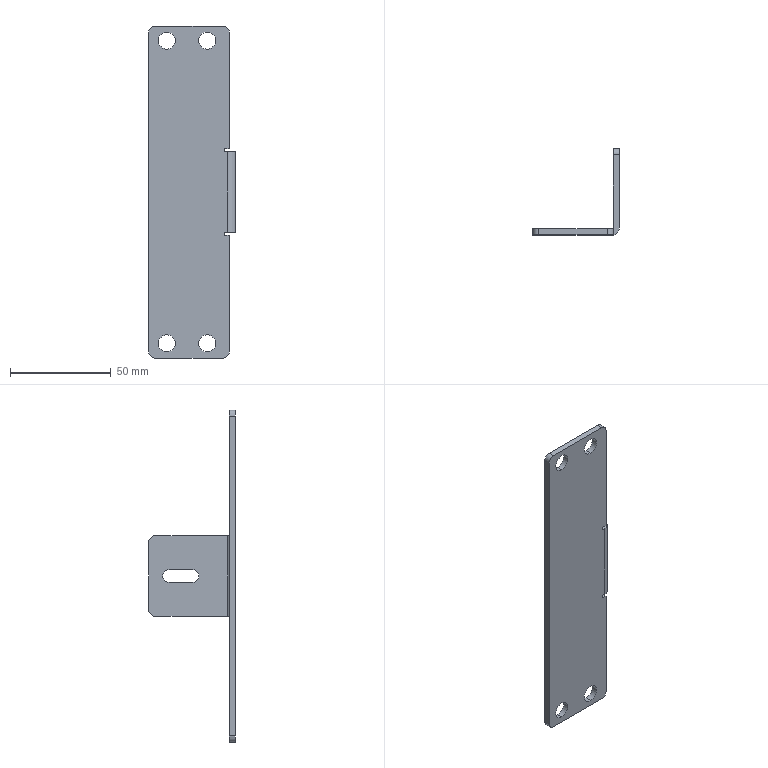Part | SolidWorks | features BaseBody 1 | 1 solid | 37 faces | box 43 x 43 x 165 mm | volume 23785 mm3 | cylinder 19 | plane 18 | commonest cylinder face diameters 8.5 x8 6 x6 6.5 x3 1.473 x1 7.473 x1
STEP:
#1=CARTESIAN_POINT('',(-11.,-3.,71.));
#2=VERTEX_POINT('',#1);
#3=CARTESIAN_POINT('',(-11.,-3.,79.5));
#4=VERTEX_POINT('',#3);
#5=CARTESIAN_POINT('',(-11.,-3.,75.25));
#6=DIRECTION('',(0.,1.,0.));
#7=DIRECTION('',(0.,0.,1.));
#8=AXIS2_PLACEMENT_3D('',#5,#6,#7);
#9=CIRCLE('',#8,4.25);
#10=EDGE_CURVE('',#2,#4,#9,.T.);
#11=ORIENTED_EDGE('',*,*,#10,.F.);
#12=CARTESIAN_POINT('',(-11.,0.,71.));
#13=VERTEX_POINT('',#12);
#14=CARTESIAN_POINT('',(-11.,-10.,71.));
#15=DIRECTION('',(0.,1.,0.));
#16=VECTOR('',#15,1000.);
#17=LINE('',#14,#16);
#18=EDGE_CURVE('',#2,#13,#17,.T.);
#19=ORIENTED_EDGE('',*,*,#18,.T.);
#20=CARTESIAN_POINT('',(-11.,0.,79.5));
#21=VERTEX_POINT('',#20);
#22=CARTESIAN_POINT('',(-11.,0.,75.25));
#23=DIRECTION('',(0.,1.,0.));
#24=DIRECTION('',(0.,0.,1.));
#25=AXIS2_PLACEMENT_3D('',#22,#23,#24);
#26=CIRCLE('',#25,4.25);
#27=EDGE_CURVE('',#13,#21,#26,.T.);
#28=ORIENTED_EDGE('',*,*,#27,.T.);
#29=CARTESIAN_POINT('',(-11.,-10.,79.5));
#30=DIRECTION('',(0.,1.,0.));
#31=VECTOR('',#30,1000.);
#32=LINE('',#29,#31);
#33=EDGE_CURVE('',#4,#21,#32,.T.);
#34=ORIENTED_EDGE('',*,*,#33,.F.);
#35=EDGE_LOOP('',(#11,#19,#28,#34));
#36=FACE_OUTER_BOUND('',#35,.T.);
#37=CARTESIAN_POINT('',(-11.,-10.,75.25));
#38=DIRECTION('',(0.,1.,0.));
#39=DIRECTION('',(0.,0.,1.));
#40=AXIS2_PLACEMENT_3D('',#37,#38,#39);
#41=CYLINDRICAL_SURFACE('',#40,4.25);
#42=ADVANCED_FACE('',(#36),#41,.F.);
#43=CARTESIAN_POINT('',(9.,-3.,71.));
#44=VERTEX_POINT('',#43);
#45=CARTESIAN_POINT('',(9.,-3.,79.5));
#46=VERTEX_POINT('',#45);
#47=CARTESIAN_POINT('',(9.,-3.,75.25));
#48=DIRECTION('',(0.,1.,0.));
#49=DIRECTION('',(0.,0.,1.));
#50=AXIS2_PLACEMENT_3D('',#47,#48,#49);
#51=CIRCLE('',#50,4.25);
#52=EDGE_CURVE('',#44,#46,#51,.T.);
#53=ORIENTED_EDGE('',*,*,#52,.F.);
#54=CARTESIAN_POINT('',(9.,0.,71.));
#55=VERTEX_POINT('',#54);
#56=CARTESIAN_POINT('',(9.,-10.,71.));
#57=DIRECTION('',(0.,1.,0.));
#58=VECTOR('',#57,1000.);
#59=LINE('',#56,#58);
#60=EDGE_CURVE('',#44,#55,#59,.T.);
#61=ORIENTED_EDGE('',*,*,#60,.T.);
#62=CARTESIAN_POINT('',(9.,0.,79.5));
#63=VERTEX_POINT('',#62);
#64=CARTESIAN_POINT('',(9.,0.,75.25));
#65=DIRECTION('',(0.,1.,0.));
#66=DIRECTION('',(0.,0.,1.));
#67=AXIS2_PLACEMENT_3D('',#64,#65,#66);
#68=CIRCLE('',#67,4.25);
#69=EDGE_CURVE('',#55,#63,#68,.T.);
#70=ORIENTED_EDGE('',*,*,#69,.T.);
#71=CARTESIAN_POINT('',(9.,-10.,79.5));
#72=DIRECTION('',(0.,1.,0.));
#73=VECTOR('',#72,1000.);
#74=LINE('',#71,#73);
#75=EDGE_CURVE('',#46,#63,#74,.T.);
#76=ORIENTED_EDGE('',*,*,#75,.F.);
#77=EDGE_LOOP('',(#53,#61,#70,#76));
#78=FACE_OUTER_BOUND('',#77,.T.);
#79=CARTESIAN_POINT('',(9.,-10.,75.25));
#80=DIRECTION('',(0.,1.,0.));
#81=DIRECTION('',(0.,0.,1.));
#82=AXIS2_PLACEMENT_3D('',#79,#80,#81);
#83=CYLINDRICAL_SURFACE('',#82,4.25);
#84=ADVANCED_FACE('',(#78),#83,.F.);
#85=CARTESIAN_POINT('',(9.,-3.,-79.5));
#86=VERTEX_POINT('',#85);
#87=CARTESIAN_POINT('',(9.,-3.,-71.));
#88=VERTEX_POINT('',#87);
#89=CARTESIAN_POINT('',(9.,-3.,-75.25));
#90=DIRECTION('',(0.,1.,0.));
#91=DIRECTION('',(0.,0.,1.));
#92=AXIS2_PLACEMENT_3D('',#89,#90,#91);
#93=CIRCLE('',#92,4.25);
#94=EDGE_CURVE('',#86,#88,#93,.T.);
#95=ORIENTED_EDGE('',*,*,#94,.F.);
#96=CARTESIAN_POINT('',(9.,0.,-79.5));
#97=VERTEX_POINT('',#96);
#98=CARTESIAN_POINT('',(9.,-10.,-79.5));
#99=DIRECTION('',(0.,1.,0.));
#100=VECTOR('',#99,1000.);
#101=LINE('',#98,#100);
#102=EDGE_CURVE('',#86,#97,#101,.T.);
#103=ORIENTED_EDGE('',*,*,#102,.T.);
#104=CARTESIAN_POINT('',(9.,0.,-71.));
#105=VERTEX_POINT('',#104);
#106=CARTESIAN_POINT('',(9.,0.,-75.25));
#107=DIRECTION('',(0.,1.,0.));
#108=DIRECTION('',(0.,0.,1.));
#109=AXIS2_PLACEMENT_3D('',#106,#107,#108);
#110=CIRCLE('',#109,4.25);
#111=EDGE_CURVE('',#97,#105,#110,.T.);
#112=ORIENTED_EDGE('',*,*,#111,.T.);
#113=CARTESIAN_POINT('',(9.,-10.,-71.));
#114=DIRECTION('',(0.,1.,0.));
#115=VECTOR('',#114,1000.);
#116=LINE('',#113,#115);
#117=EDGE_CURVE('',#88,#105,#116,.T.);
#118=ORIENTED_EDGE('',*,*,#117,.F.);
#119=EDGE_LOOP('',(#95,#103,#112,#118));
#120=FACE_OUTER_BOUND('',#119,.T.);
#121=CARTESIAN_POINT('',(9.,-10.,-75.25));
#122=DIRECTION('',(0.,1.,0.));
#123=DIRECTION('',(0.,0.,1.));
#124=AXIS2_PLACEMENT_3D('',#121,#122,#123);
#125=CYLINDRICAL_SURFACE('',#124,4.25);
#126=ADVANCED_FACE('',(#120),#125,.F.);
#127=CARTESIAN_POINT('',(-11.,-3.,-79.5));
#128=VERTEX_POINT('',#127);
#129=CARTESIAN_POINT('',(-11.,-3.,-71.));
#130=VERTEX_POINT('',#129);
#131=CARTESIAN_POINT('',(-11.,-3.,-75.25));
#132=DIRECTION('',(0.,1.,0.));
#133=DIRECTION('',(0.,0.,1.));
#134=AXIS2_PLACEMENT_3D('',#131,#132,#133);
#135=CIRCLE('',#134,4.25);
#136=EDGE_CURVE('',#128,#130,#135,.T.);
#137=ORIENTED_EDGE('',*,*,#136,.F.);
#138=CARTESIAN_POINT('',(-11.,0.,-79.5));
#139=VERTEX_POINT('',#138);
#140=CARTESIAN_POINT('',(-11.,-10.,-79.5));
#141=DIRECTION('',(0.,1.,0.));
#142=VECTOR('',#141,1000.);
#143=LINE('',#140,#142);
#144=EDGE_CURVE('',#128,#139,#143,.T.);
#145=ORIENTED_EDGE('',*,*,#144,.T.);
#146=CARTESIAN_POINT('',(-11.,0.,-71.));
#147=VERTEX_POINT('',#146);
#148=CARTESIAN_POINT('',(-11.,0.,-75.25));
#149=DIRECTION('',(0.,1.,0.));
#150=DIRECTION('',(0.,0.,1.));
#151=AXIS2_PLACEMENT_3D('',#148,#149,#150);
#152=CIRCLE('',#151,4.25);
#153=EDGE_CURVE('',#139,#147,#152,.T.);
#154=ORIENTED_EDGE('',*,*,#153,.T.);
#155=CARTESIAN_POINT('',(-11.,-10.,-71.));
#156=DIRECTION('',(0.,1.,0.));
#157=VECTOR('',#156,1000.);
#158=LINE('',#155,#157);
#159=EDGE_CURVE('',#130,#147,#158,.T.);
#160=ORIENTED_EDGE('',*,*,#159,.F.);
#161=EDGE_LOOP('',(#137,#145,#154,#160));
#162=FACE_OUTER_BOUND('',#161,.T.);
#163=CARTESIAN_POINT('',(-11.,-10.,-75.25));
#164=DIRECTION('',(0.,1.,0.));
#165=DIRECTION('',(0.,0.,1.));
#166=AXIS2_PLACEMENT_3D('',#163,#164,#165);
#167=CYLINDRICAL_SURFACE('',#166,4.25);
#168=ADVANCED_FACE('',(#162),#167,.F.);
#169=CARTESIAN_POINT('',(20.,33.,0.));
#170=VERTEX_POINT('',#169);
#171=CARTESIAN_POINT('',(20.,29.75,3.25));
#172=VERTEX_POINT('',#171);
#173=CARTESIAN_POINT('',(20.,29.75,0.));
#174=DIRECTION('',(1.,0.,0.));
#175=DIRECTION('',(0.,1.,0.));
#176=AXIS2_PLACEMENT_3D('',#173,#174,#175);
#177=CIRCLE('',#176,3.25);
#178=EDGE_CURVE('',#170,#172,#177,.T.);
#179=ORIENTED_EDGE('',*,*,#178,.F.);
#180=CARTESIAN_POINT('',(23.,33.,0.));
#181=VERTEX_POINT('',#180);
#182=CARTESIAN_POINT('',(13.,33.,0.));
#183=DIRECTION('',(1.,0.,0.));
#184=VECTOR('',#183,1000.);
#185=LINE('',#182,#184);
#186=EDGE_CURVE('',#170,#181,#185,.T.);
#187=ORIENTED_EDGE('',*,*,#186,.T.);
#188=CARTESIAN_POINT('',(23.,29.75,3.25));
#189=VERTEX_POINT('',#188);
#190=CARTESIAN_POINT('',(23.,29.75,0.));
#191=DIRECTION('',(-1.,0.,0.));
#192=DIRECTION('',(0.,1.,0.));
#193=AXIS2_PLACEMENT_3D('',#190,#191,#192);
#194=CIRCLE('',#193,3.25);
#195=EDGE_CURVE('',#189,#181,#194,.T.);
#196=ORIENTED_EDGE('',*,*,#195,.F.);
#197=CARTESIAN_POINT('',(13.,29.75,3.25));
#198=DIRECTION('',(-1.,0.,0.));
#199=VECTOR('',#198,1000.);
#200=LINE('',#197,#199);
#201=EDGE_CURVE('',#189,#172,#200,.T.);
#202=ORIENTED_EDGE('',*,*,#201,.T.);
#203=EDGE_LOOP('',(#179,#187,#196,#202));
#204=FACE_OUTER_BOUND('',#203,.T.);
#205=CARTESIAN_POINT('',(13.,29.75,0.));
#206=DIRECTION('',(1.,0.,0.));
#207=DIRECTION('',(0.,1.,0.));
#208=AXIS2_PLACEMENT_3D('',#205,#206,#207);
#209=CYLINDRICAL_SURFACE('',#208,3.25);
#210=ADVANCED_FACE('',(#204),#209,.F.);
#211=CARTESIAN_POINT('',(17.,0.,-82.5));
#212=VERTEX_POINT('',#211);
#213=CARTESIAN_POINT('',(20.,0.,-79.5));
#214=VERTEX_POINT('',#213);
#215=CARTESIAN_POINT('',(17.,0.,-79.5));
#216=DIRECTION('',(0.,-1.,0.));
#217=DIRECTION('',(0.,0.,1.));
#218=AXIS2_PLACEMENT_3D('',#215,#216,#217);
#219=CIRCLE('',#218,3.);
#220=EDGE_CURVE('',#212,#214,#219,.T.);
#221=ORIENTED_EDGE('',*,*,#220,.F.);
#222=CARTESIAN_POINT('',(-17.,0.,-82.5));
#223=VERTEX_POINT('',#222);
#224=CARTESIAN_POINT('',(0.,0.,-82.5));
#225=DIRECTION('',(1.,0.,0.));
#226=VECTOR('',#225,1000.);
#227=LINE('',#224,#226);
#228=EDGE_CURVE('',#223,#212,#227,.T.);
#229=ORIENTED_EDGE('',*,*,#228,.F.);
#230=CARTESIAN_POINT('',(-20.,0.,-79.5));
#231=VERTEX_POINT('',#230);
#232=CARTESIAN_POINT('',(-17.,0.,-79.5));
#233=DIRECTION('',(0.,-1.,0.));
#234=DIRECTION('',(0.,0.,1.));
#235=AXIS2_PLACEMENT_3D('',#232,#233,#234);
#236=CIRCLE('',#235,3.);
#237=EDGE_CURVE('',#231,#223,#236,.T.);
#238=ORIENTED_EDGE('',*,*,#237,.F.);
#239=CARTESIAN_POINT('',(-20.,0.,79.5));
#240=VERTEX_POINT('',#239);
#241=CARTESIAN_POINT('',(-20.,0.,0.));
#242=DIRECTION('',(0.,0.,-1.));
#243=VECTOR('',#242,1000.);
#244=LINE('',#241,#243);
#245=EDGE_CURVE('',#240,#231,#244,.T.);
#246=ORIENTED_EDGE('',*,*,#245,.F.);
#247=CARTESIAN_POINT('',(-17.,0.,82.5));
#248=VERTEX_POINT('',#247);
#249=CARTESIAN_POINT('',(-17.,0.,79.5));
#250=DIRECTION('',(0.,-1.,0.));
#251=DIRECTION('',(0.,0.,1.));
#252=AXIS2_PLACEMENT_3D('',#249,#250,#251);
#253=CIRCLE('',#252,3.);
#254=EDGE_CURVE('',#248,#240,#253,.T.);
#255=ORIENTED_EDGE('',*,*,#254,.F.);
#256=CARTESIAN_POINT('',(17.,0.,82.5));
#257=VERTEX_POINT('',#256);
#258=CARTESIAN_POINT('',(0.,0.,82.5));
#259=DIRECTION('',(-1.,0.,0.));
#260=VECTOR('',#259,1000.);
#261=LINE('',#258,#260);
#262=EDGE_CURVE('',#257,#248,#261,.T.);
#263=ORIENTED_EDGE('',*,*,#262,.F.);
#264=CARTESIAN_POINT('',(20.,0.,79.5));
#265=VERTEX_POINT('',#264);
#266=CARTESIAN_POINT('',(17.,0.,79.5));
#267=DIRECTION('',(0.,-1.,0.));
#268=DIRECTION('',(0.,0.,1.));
#269=AXIS2_PLACEMENT_3D('',#266,#267,#268);
#270=CIRCLE('',#269,3.);
#271=EDGE_CURVE('',#265,#257,#270,.T.);
#272=ORIENTED_EDGE('',*,*,#271,.F.);
#273=CARTESIAN_POINT('',(20.,0.,21.5));
#274=VERTEX_POINT('',#273);
#275=CARTESIAN_POINT('',(20.,0.,0.));
#276=DIRECTION('',(0.,0.,1.));
#277=VECTOR('',#276,1000.);
#278=LINE('',#275,#277);
#279=EDGE_CURVE('',#274,#265,#278,.T.);
#280=ORIENTED_EDGE('',*,*,#279,.F.);
#281=CARTESIAN_POINT('',(17.763,0.,21.5));
#282=VERTEX_POINT('',#281);
#283=CARTESIAN_POINT('',(0.,0.,21.5));
#284=DIRECTION('',(1.,0.,0.));
#285=VECTOR('',#284,1000.);
#286=LINE('',#283,#285);
#287=EDGE_CURVE('',#282,#274,#286,.T.);
#288=ORIENTED_EDGE('',*,*,#287,.F.);
#289=CARTESIAN_POINT('',(17.763,0.,20.));
#290=VERTEX_POINT('',#289);
#291=CARTESIAN_POINT('',(17.763,0.,20.));
#292=DIRECTION('',(0.,0.,1.));
#293=VECTOR('',#292,1000.);
#294=LINE('',#291,#293);
#295=EDGE_CURVE('',#290,#282,#294,.T.);
#296=ORIENTED_EDGE('',*,*,#295,.F.);
#297=CARTESIAN_POINT('',(19.263,0.,20.));
#298=VERTEX_POINT('',#297);
#299=CARTESIAN_POINT('',(19.263,0.,20.));
#300=DIRECTION('',(-1.,0.,0.));
#301=VECTOR('',#300,1000.);
#302=LINE('',#299,#301);
#303=EDGE_CURVE('',#298,#290,#302,.T.);
#304=ORIENTED_EDGE('',*,*,#303,.F.);
#305=CARTESIAN_POINT('',(19.263,0.,-20.));
#306=VERTEX_POINT('',#305);
#307=CARTESIAN_POINT('',(19.263,0.,0.));
#308=DIRECTION('',(0.,0.,1.));
#309=VECTOR('',#308,1000.);
#310=LINE('',#307,#309);
#311=EDGE_CURVE('',#306,#298,#310,.T.);
#312=ORIENTED_EDGE('',*,*,#311,.F.);
#313=CARTESIAN_POINT('',(17.763,0.,-20.));
#314=VERTEX_POINT('',#313);
#315=CARTESIAN_POINT('',(17.763,0.,-20.));
#316=DIRECTION('',(1.,0.,0.));
#317=VECTOR('',#316,1000.);
#318=LINE('',#315,#317);
#319=EDGE_CURVE('',#314,#306,#318,.T.);
#320=ORIENTED_EDGE('',*,*,#319,.F.);
#321=CARTESIAN_POINT('',(17.763,0.,-21.5));
#322=VERTEX_POINT('',#321);
#323=CARTESIAN_POINT('',(17.763,0.,-21.5));
#324=DIRECTION('',(0.,0.,1.));
#325=VECTOR('',#324,1000.);
#326=LINE('',#323,#325);
#327=EDGE_CURVE('',#322,#314,#326,.T.);
#328=ORIENTED_EDGE('',*,*,#327,.F.);
#329=CARTESIAN_POINT('',(20.,0.,-21.5));
#330=VERTEX_POINT('',#329);
#331=CARTESIAN_POINT('',(0.,0.,-21.5));
#332=DIRECTION('',(-1.,0.,0.));
#333=VECTOR('',#332,1000.);
#334=LINE('',#331,#333);
#335=EDGE_CURVE('',#330,#322,#334,.T.);
#336=ORIENTED_EDGE('',*,*,#335,.F.);
#337=CARTESIAN_POINT('',(20.,0.,0.));
#338=DIRECTION('',(0.,0.,1.));
#339=VECTOR('',#338,1000.);
#340=LINE('',#337,#339);
#341=EDGE_CURVE('',#214,#330,#340,.T.);
#342=ORIENTED_EDGE('',*,*,#341,.F.);
#343=EDGE_LOOP('',(#221,#229,#238,#246,#255,#263,#272,#280,#288,#296,#304,#312,#320,#328,#336,#342));
#344=FACE_OUTER_BOUND('',#343,.T.);
#345=CARTESIAN_POINT('',(-11.,0.,75.25));
#346=DIRECTION('',(0.,1.,0.));
#347=DIRECTION('',(0.,0.,1.));
#348=AXIS2_PLACEMENT_3D('',#345,#346,#347);
#349=CIRCLE('',#348,4.25);
#350=EDGE_CURVE('',#21,#13,#349,.T.);
#351=ORIENTED_EDGE('',*,*,#350,.F.);
#352=ORIENTED_EDGE('',*,*,#27,.F.);
#353=EDGE_LOOP('',(#351,#352));
#354=FACE_BOUND('',#353,.T.);
#355=CARTESIAN_POINT('',(9.,0.,75.25));
#356=DIRECTION('',(0.,1.,0.));
#357=DIRECTION('',(0.,0.,1.));
#358=AXIS2_PLACEMENT_3D('',#355,#356,#357);
#359=CIRCLE('',#358,4.25);
#360=EDGE_CURVE('',#63,#55,#359,.T.);
#361=ORIENTED_EDGE('',*,*,#360,.F.);
#362=ORIENTED_EDGE('',*,*,#69,.F.);
#363=EDGE_LOOP('',(#361,#362));
#364=FACE_BOUND('',#363,.T.);
#365=CARTESIAN_POINT('',(9.,0.,-75.25));
#366=DIRECTION('',(0.,1.,0.));
#367=DIRECTION('',(0.,0.,1.));
#368=AXIS2_PLACEMENT_3D('',#365,#366,#367);
#369=CIRCLE('',#368,4.25);
#370=EDGE_CURVE('',#105,#97,#369,.T.);
#371=ORIENTED_EDGE('',*,*,#370,.F.);
#372=ORIENTED_EDGE('',*,*,#111,.F.);
#373=EDGE_LOOP('',(#371,#372));
#374=FACE_BOUND('',#373,.T.);
#375=CARTESIAN_POINT('',(-11.,0.,-75.25));
#376=DIRECTION('',(0.,1.,0.));
#377=DIRECTION('',(0.,0.,1.));
#378=AXIS2_PLACEMENT_3D('',#375,#376,#377);
#379=CIRCLE('',#378,4.25);
#380=EDGE_CURVE('',#147,#139,#379,.T.);
#381=ORIENTED_EDGE('',*,*,#380,.F.);
#382=ORIENTED_EDGE('',*,*,#153,.F.);
#383=EDGE_LOOP('',(#381,#382));
#384=FACE_BOUND('',#383,.T.);
#385=CARTESIAN_POINT('',(0.,0.,0.));
#386=DIRECTION('',(0.,-1.,0.));
#387=DIRECTION('',(0.,0.,-1.));
#388=AXIS2_PLACEMENT_3D('',#385,#386,#387);
#389=PLANE('',#388);
#390=ADVANCED_FACE('',(#344,#354,#364,#374,#384),#389,.F.);
#391=ORIENTED_EDGE('',*,*,#341,.T.);
#392=CARTESIAN_POINT('',(20.,-3.,-21.5));
#393=VERTEX_POINT('',#392);
#394=CARTESIAN_POINT('',(20.,-3.,-21.5));
#395=DIRECTION('',(0.,-1.,0.));
#396=VECTOR('',#395,1000.);
#397=LINE('',#394,#396);
#398=EDGE_CURVE('',#330,#393,#397,.T.);
#399=ORIENTED_EDGE('',*,*,#398,.T.);
#400=CARTESIAN_POINT('',(20.,-3.,-79.5));
#401=VERTEX_POINT('',#400);
#402=CARTESIAN_POINT('',(20.,-3.,82.5));
#403=DIRECTION('',(0.,0.,-1.));
#404=VECTOR('',#403,1000.);
#405=LINE('',#402,#404);
#406=EDGE_CURVE('',#393,#401,#405,.T.);
#407=ORIENTED_EDGE('',*,*,#406,.T.);
#408=CARTESIAN_POINT('',(20.,-3.,-79.5));
#409=DIRECTION('',(0.,1.,0.));
#410=VECTOR('',#409,1000.);
#411=LINE('',#408,#410);
#412=EDGE_CURVE('',#401,#214,#411,.T.);
#413=ORIENTED_EDGE('',*,*,#412,.T.);
#414=EDGE_LOOP('',(#391,#399,#407,#413));
#415=FACE_OUTER_BOUND('',#414,.T.);
#416=CARTESIAN_POINT('',(20.,-3.,82.5));
#417=DIRECTION('',(1.,0.,0.));
#418=DIRECTION('',(0.,0.,-1.));
#419=AXIS2_PLACEMENT_3D('',#416,#417,#418);
#420=PLANE('',#419);
#421=ADVANCED_FACE('',(#415),#420,.T.);
#422=ORIENTED_EDGE('',*,*,#220,.T.);
#423=ORIENTED_EDGE('',*,*,#412,.F.);
#424=CARTESIAN_POINT('',(17.,-3.,-82.5));
#425=VERTEX_POINT('',#424);
#426=CARTESIAN_POINT('',(17.,-3.,-79.5));
#427=DIRECTION('',(0.,1.,0.));
#428=DIRECTION('',(0.,0.,1.));
#429=AXIS2_PLACEMENT_3D('',#426,#427,#428);
#430=CIRCLE('',#429,3.);
#431=EDGE_CURVE('',#401,#425,#430,.T.);
#432=ORIENTED_EDGE('',*,*,#431,.T.);
#433=CARTESIAN_POINT('',(17.,-3.,-82.5));
#434=DIRECTION('',(0.,1.,0.));
#435=VECTOR('',#434,1000.);
#436=LINE('',#433,#435);
#437=EDGE_CURVE('',#425,#212,#436,.T.);
#438=ORIENTED_EDGE('',*,*,#437,.T.);
#439=EDGE_LOOP('',(#422,#423,#432,#438));
#440=FACE_OUTER_BOUND('',#439,.T.);
#441=CARTESIAN_POINT('',(17.,-3.,-79.5));
#442=DIRECTION('',(0.,1.,0.));
#443=DIRECTION('',(0.,0.,1.));
#444=AXIS2_PLACEMENT_3D('',#441,#442,#443);
#445=CYLINDRICAL_SURFACE('',#444,3.);
#446=ADVANCED_FACE('',(#440),#445,.T.);
#447=CARTESIAN_POINT('',(-17.,-3.,-82.5));
#448=VERTEX_POINT('',#447);
#449=CARTESIAN_POINT('',(-20.,-3.,-82.5));
#450=DIRECTION('',(-1.,0.,0.));
#451=VECTOR('',#450,1000.);
#452=LINE('',#449,#451);
#453=EDGE_CURVE('',#425,#448,#452,.T.);
#454=ORIENTED_EDGE('',*,*,#453,.T.);
#455=CARTESIAN_POINT('',(-17.,-3.,-82.5));
#456=DIRECTION('',(0.,1.,0.));
#457=VECTOR('',#456,1000.);
#458=LINE('',#455,#457);
#459=EDGE_CURVE('',#448,#223,#458,.T.);
#460=ORIENTED_EDGE('',*,*,#459,.T.);
#461=ORIENTED_EDGE('',*,*,#228,.T.);
#462=ORIENTED_EDGE('',*,*,#437,.F.);
#463=EDGE_LOOP('',(#454,#460,#461,#462));
#464=FACE_OUTER_BOUND('',#463,.T.);
#465=CARTESIAN_POINT('',(-20.,-3.,-82.5));
#466=DIRECTION('',(0.,0.,-1.));
#467=DIRECTION('',(-1.,0.,0.));
#468=AXIS2_PLACEMENT_3D('',#465,#466,#467);
#469=PLANE('',#468);
#470=ADVANCED_FACE('',(#464),#469,.T.);
#471=ORIENTED_EDGE('',*,*,#237,.T.);
#472=ORIENTED_EDGE('',*,*,#459,.F.);
#473=CARTESIAN_POINT('',(-20.,-3.,-79.5));
#474=VERTEX_POINT('',#473);
#475=CARTESIAN_POINT('',(-17.,-3.,-79.5));
#476=DIRECTION('',(0.,1.,0.));
#477=DIRECTION('',(0.,0.,1.));
#478=AXIS2_PLACEMENT_3D('',#475,#476,#477);
#479=CIRCLE('',#478,3.);
#480=EDGE_CURVE('',#448,#474,#479,.T.);
#481=ORIENTED_EDGE('',*,*,#480,.T.);
#482=CARTESIAN_POINT('',(-20.,-3.,-79.5));
#483=DIRECTION('',(0.,1.,0.));
#484=VECTOR('',#483,1000.);
#485=LINE('',#482,#484);
#486=EDGE_CURVE('',#474,#231,#485,.T.);
#487=ORIENTED_EDGE('',*,*,#486,.T.);
#488=EDGE_LOOP('',(#471,#472,#481,#487));
#489=FACE_OUTER_BOUND('',#488,.T.);
#490=CARTESIAN_POINT('',(-17.,-3.,-79.5));
#491=DIRECTION('',(0.,1.,0.));
#492=DIRECTION('',(0.,0.,1.));
#493=AXIS2_PLACEMENT_3D('',#490,#491,#492);
#494=CYLINDRICAL_SURFACE('',#493,3.);
#495=ADVANCED_FACE('',(#489),#494,.T.);
#496=CARTESIAN_POINT('',(-20.,-3.,79.5));
#497=VERTEX_POINT('',#496);
#498=CARTESIAN_POINT('',(-20.,-3.,82.5));
#499=DIRECTION('',(0.,0.,1.));
#500=VECTOR('',#499,1000.);
#501=LINE('',#498,#500);
#502=EDGE_CURVE('',#474,#497,#501,.T.);
#503=ORIENTED_EDGE('',*,*,#502,.T.);
#504=CARTESIAN_POINT('',(-20.,-3.,79.5));
#505=DIRECTION('',(0.,1.,0.));
#506=VECTOR('',#505,1000.);
#507=LINE('',#504,#506);
#508=EDGE_CURVE('',#497,#240,#507,.T.);
#509=ORIENTED_EDGE('',*,*,#508,.T.);
#510=ORIENTED_EDGE('',*,*,#245,.T.);
#511=ORIENTED_EDGE('',*,*,#486,.F.);
#512=EDGE_LOOP('',(#503,#509,#510,#511));
#513=FACE_OUTER_BOUND('',#512,.T.);
#514=CARTESIAN_POINT('',(-20.,-3.,82.5));
#515=DIRECTION('',(-1.,0.,0.));
#516=DIRECTION('',(0.,0.,1.));
#517=AXIS2_PLACEMENT_3D('',#514,#515,#516);
#518=PLANE('',#517);
#519=ADVANCED_FACE('',(#513),#518,.T.);
#520=ORIENTED_EDGE('',*,*,#254,.T.);
#521=ORIENTED_EDGE('',*,*,#508,.F.);
#522=CARTESIAN_POINT('',(-17.,-3.,82.5));
#523=VERTEX_POINT('',#522);
#524=CARTESIAN_POINT('',(-17.,-3.,79.5));
#525=DIRECTION('',(0.,1.,0.));
#526=DIRECTION('',(0.,0.,1.));
#527=AXIS2_PLACEMENT_3D('',#524,#525,#526);
#528=CIRCLE('',#527,3.);
#529=EDGE_CURVE('',#497,#523,#528,.T.);
#530=ORIENTED_EDGE('',*,*,#529,.T.);
#531=CARTESIAN_POINT('',(-17.,-3.,82.5));
#532=DIRECTION('',(0.,1.,0.));
#533=VECTOR('',#532,1000.);
#534=LINE('',#531,#533);
#535=EDGE_CURVE('',#523,#248,#534,.T.);
#536=ORIENTED_EDGE('',*,*,#535,.T.);
#537=EDGE_LOOP('',(#520,#521,#530,#536));
#538=FACE_OUTER_BOUND('',#537,.T.);
#539=CARTESIAN_POINT('',(-17.,-3.,79.5));
#540=DIRECTION('',(0.,1.,0.));
#541=DIRECTION('',(0.,0.,1.));
#542=AXIS2_PLACEMENT_3D('',#539,#540,#541);
#543=CYLINDRICAL_SURFACE('',#542,3.);
#544=ADVANCED_FACE('',(#538),#543,.T.);
#545=CARTESIAN_POINT('',(17.,-3.,82.5));
#546=VERTEX_POINT('',#545);
#547=CARTESIAN_POINT('',(-20.,-3.,82.5));
#548=DIRECTION('',(1.,0.,0.));
#549=VECTOR('',#548,1000.);
#550=LINE('',#547,#549);
#551=EDGE_CURVE('',#523,#546,#550,.T.);
#552=ORIENTED_EDGE('',*,*,#551,.T.);
#553=CARTESIAN_POINT('',(17.,-3.,82.5));
#554=DIRECTION('',(0.,1.,0.));
#555=VECTOR('',#554,1000.);
#556=LINE('',#553,#555);
#557=EDGE_CURVE('',#546,#257,#556,.T.);
#558=ORIENTED_EDGE('',*,*,#557,.T.);
#559=ORIENTED_EDGE('',*,*,#262,.T.);
#560=ORIENTED_EDGE('',*,*,#535,.F.);
#561=EDGE_LOOP('',(#552,#558,#559,#560));
#562=FACE_OUTER_BOUND('',#561,.T.);
#563=CARTESIAN_POINT('',(-20.,-3.,82.5));
#564=DIRECTION('',(0.,0.,1.));
#565=DIRECTION('',(1.,0.,0.));
#566=AXIS2_PLACEMENT_3D('',#563,#564,#565);
#567=PLANE('',#566);
#568=ADVANCED_FACE('',(#562),#567,.T.);
#569=ORIENTED_EDGE('',*,*,#271,.T.);
#570=ORIENTED_EDGE('',*,*,#557,.F.);
#571=CARTESIAN_POINT('',(20.,-3.,79.5));
#572=VERTEX_POINT('',#571);
#573=CARTESIAN_POINT('',(17.,-3.,79.5));
#574=DIRECTION('',(0.,1.,0.));
#575=DIRECTION('',(0.,0.,1.));
#576=AXIS2_PLACEMENT_3D('',#573,#574,#575);
#577=CIRCLE('',#576,3.);
#578=EDGE_CURVE('',#546,#572,#577,.T.);
#579=ORIENTED_EDGE('',*,*,#578,.T.);
#580=CARTESIAN_POINT('',(20.,-3.,79.5));
#581=DIRECTION('',(0.,1.,0.));
#582=VECTOR('',#581,1000.);
#583=LINE('',#580,#582);
#584=EDGE_CURVE('',#572,#265,#583,.T.);
#585=ORIENTED_EDGE('',*,*,#584,.T.);
#586=EDGE_LOOP('',(#569,#570,#579,#585));
#587=FACE_OUTER_BOUND('',#586,.T.);
#588=CARTESIAN_POINT('',(17.,-3.,79.5));
#589=DIRECTION('',(0.,1.,0.));
#590=DIRECTION('',(0.,0.,1.));
#591=AXIS2_PLACEMENT_3D('',#588,#589,#590);
#592=CYLINDRICAL_SURFACE('',#591,3.);
#593=ADVANCED_FACE('',(#587),#592,.T.);
#594=CARTESIAN_POINT('',(20.,-3.,21.5));
#595=VERTEX_POINT('',#594);
#596=CARTESIAN_POINT('',(20.,-3.,82.5));
#597=DIRECTION('',(0.,0.,-1.));
#598=VECTOR('',#597,1000.);
#599=LINE('',#596,#598);
#600=EDGE_CURVE('',#572,#595,#599,.T.);
#601=ORIENTED_EDGE('',*,*,#600,.T.);
#602=CARTESIAN_POINT('',(20.,-3.,21.5));
#603=DIRECTION('',(0.,1.,0.));
#604=VECTOR('',#603,1000.);
#605=LINE('',#602,#604);
#606=EDGE_CURVE('',#595,#274,#605,.T.);
#607=ORIENTED_EDGE('',*,*,#606,.T.);
#608=ORIENTED_EDGE('',*,*,#279,.T.);
#609=ORIENTED_EDGE('',*,*,#584,.F.);
#610=EDGE_LOOP('',(#601,#607,#608,#609));
#611=FACE_OUTER_BOUND('',#610,.T.);
#612=CARTESIAN_POINT('',(20.,-3.,82.5));
#613=DIRECTION('',(1.,0.,0.));
#614=DIRECTION('',(0.,0.,-1.));
#615=AXIS2_PLACEMENT_3D('',#612,#613,#614);
#616=PLANE('',#615);
#617=ADVANCED_FACE('',(#611),#616,.T.);
#618=ORIENTED_EDGE('',*,*,#287,.T.);
#619=ORIENTED_EDGE('',*,*,#606,.F.);
#620=CARTESIAN_POINT('',(17.763,-3.,21.5));
#621=VERTEX_POINT('',#620);
#622=CARTESIAN_POINT('',(17.763,-3.,21.5));
#623=DIRECTION('',(-1.,0.,0.));
#624=VECTOR('',#623,1000.);
#625=LINE('',#622,#624);
#626=EDGE_CURVE('',#595,#621,#625,.T.);
#627=ORIENTED_EDGE('',*,*,#626,.T.);
#628=CARTESIAN_POINT('',(17.763,0.,21.5));
#629=DIRECTION('',(0.,1.,0.));
#630=VECTOR('',#629,1000.);
#631=LINE('',#628,#630);
#632=EDGE_CURVE('',#621,#282,#631,.T.);
#633=ORIENTED_EDGE('',*,*,#632,.T.);
#634=EDGE_LOOP('',(#618,#619,#627,#633));
#635=FACE_OUTER_BOUND('',#634,.T.);
#636=CARTESIAN_POINT('',(17.763,0.,21.5));
#637=DIRECTION('',(0.,0.,-1.));
#638=DIRECTION('',(-1.,0.,0.));
#639=AXIS2_PLACEMENT_3D('',#636,#637,#638);
#640=PLANE('',#639);
#641=ADVANCED_FACE('',(#635),#640,.T.);
#642=CARTESIAN_POINT('',(20.,0.7366,20.));
#643=VERTEX_POINT('',#642);
#644=CARTESIAN_POINT('',(19.263,0.7366,20.));
#645=DIRECTION('',(0.,0.,-1.));
#646=DIRECTION('',(-1.,0.,0.));
#647=AXIS2_PLACEMENT_3D('',#644,#645,#646);
#648=CIRCLE('',#647,0.7366);
#649=EDGE_CURVE('',#643,#298,#648,.T.);
#650=ORIENTED_EDGE('',*,*,#649,.F.);
#651=CARTESIAN_POINT('',(20.,0.7366,-20.));
#652=VERTEX_POINT('',#651);
#653=CARTESIAN_POINT('',(20.,0.7366,-20.));
#654=DIRECTION('',(0.,0.,1.));
#655=VECTOR('',#654,1000.);
#656=LINE('',#653,#655);
#657=EDGE_CURVE('',#652,#643,#656,.T.);
#658=ORIENTED_EDGE('',*,*,#657,.F.);
#659=CARTESIAN_POINT('',(19.263,0.7366,-20.));
#660=DIRECTION('',(0.,0.,-1.));
#661=DIRECTION('',(-1.,0.,0.));
#662=AXIS2_PLACEMENT_3D('',#659,#660,#661);
#663=CIRCLE('',#662,0.7366);
#664=EDGE_CURVE('',#652,#306,#663,.T.);
#665=ORIENTED_EDGE('',*,*,#664,.T.);
#666=ORIENTED_EDGE('',*,*,#311,.T.);
#667=EDGE_LOOP('',(#650,#658,#665,#666));
#668=FACE_OUTER_BOUND('',#667,.T.);
#669=CARTESIAN_POINT('',(19.263,0.7366,-20.));
#670=DIRECTION('',(0.,0.,-1.));
#671=DIRECTION('',(-1.,0.,0.));
#672=AXIS2_PLACEMENT_3D('',#669,#670,#671);
#673=CYLINDRICAL_SURFACE('',#672,0.7366);
#674=ADVANCED_FACE('',(#668),#673,.F.);
#675=ORIENTED_EDGE('',*,*,#335,.T.);
#676=CARTESIAN_POINT('',(17.763,-3.,-21.5));
#677=VERTEX_POINT('',#676);
#678=CARTESIAN_POINT('',(17.763,0.,-21.5));
#679=DIRECTION('',(0.,-1.,0.));
#680=VECTOR('',#679,1000.);
#681=LINE('',#678,#680);
#682=EDGE_CURVE('',#322,#677,#681,.T.);
#683=ORIENTED_EDGE('',*,*,#682,.T.);
#684=CARTESIAN_POINT('',(20.,-3.,-21.5));
#685=DIRECTION('',(1.,0.,0.));
#686=VECTOR('',#685,1000.);
#687=LINE('',#684,#686);
#688=EDGE_CURVE('',#677,#393,#687,.T.);
#689=ORIENTED_EDGE('',*,*,#688,.T.);
#690=ORIENTED_EDGE('',*,*,#398,.F.);
#691=EDGE_LOOP('',(#675,#683,#689,#690));
#692=FACE_OUTER_BOUND('',#691,.T.);
#693=CARTESIAN_POINT('',(20.,0.,-21.5));
#694=DIRECTION('',(0.,0.,1.));
#695=DIRECTION('',(1.,0.,0.));
#696=AXIS2_PLACEMENT_3D('',#693,#694,#695);
#697=PLANE('',#696);
#698=ADVANCED_FACE('',(#692),#697,.T.);
#699=ORIENTED_EDGE('',*,*,#18,.F.);
#700=CARTESIAN_POINT('',(-11.,-3.,75.25));
#701=DIRECTION('',(0.,1.,0.));
#702=DIRECTION('',(0.,0.,1.));
#703=AXIS2_PLACEMENT_3D('',#700,#701,#702);
#704=CIRCLE('',#703,4.25);
#705=EDGE_CURVE('',#4,#2,#704,.T.);
#706=ORIENTED_EDGE('',*,*,#705,.F.);
#707=ORIENTED_EDGE('',*,*,#33,.T.);
#708=ORIENTED_EDGE('',*,*,#350,.T.);
#709=EDGE_LOOP('',(#699,#706,#707,#708));
#710=FACE_OUTER_BOUND('',#709,.T.);
#711=CARTESIAN_POINT('',(-11.,-10.,75.25));
#712=DIRECTION('',(0.,1.,0.));
#713=DIRECTION('',(0.,0.,1.));
#714=AXIS2_PLACEMENT_3D('',#711,#712,#713);
#715=CYLINDRICAL_SURFACE('',#714,4.25);
#716=ADVANCED_FACE('',(#710),#715,.F.);
#717=ORIENTED_EDGE('',*,*,#60,.F.);
#718=CARTESIAN_POINT('',(9.,-3.,75.25));
#719=DIRECTION('',(0.,1.,0.));
#720=DIRECTION('',(0.,0.,1.));
#721=AXIS2_PLACEMENT_3D('',#718,#719,#720);
#722=CIRCLE('',#721,4.25);
#723=EDGE_CURVE('',#46,#44,#722,.T.);
#724=ORIENTED_EDGE('',*,*,#723,.F.);
#725=ORIENTED_EDGE('',*,*,#75,.T.);
#726=ORIENTED_EDGE('',*,*,#360,.T.);
#727=EDGE_LOOP('',(#717,#724,#725,#726));
#728=FACE_OUTER_BOUND('',#727,.T.);
#729=CARTESIAN_POINT('',(9.,-10.,75.25));
#730=DIRECTION('',(0.,1.,0.));
#731=DIRECTION('',(0.,0.,1.));
#732=AXIS2_PLACEMENT_3D('',#729,#730,#731);
#733=CYLINDRICAL_SURFACE('',#732,4.25);
#734=ADVANCED_FACE('',(#728),#733,.F.);
#735=ORIENTED_EDGE('',*,*,#102,.F.);
#736=CARTESIAN_POINT('',(9.,-3.,-75.25));
#737=DIRECTION('',(0.,1.,0.));
#738=DIRECTION('',(0.,0.,1.));
#739=AXIS2_PLACEMENT_3D('',#736,#737,#738);
#740=CIRCLE('',#739,4.25);
#741=EDGE_CURVE('',#88,#86,#740,.T.);
#742=ORIENTED_EDGE('',*,*,#741,.F.);
#743=ORIENTED_EDGE('',*,*,#117,.T.);
#744=ORIENTED_EDGE('',*,*,#370,.T.);
#745=EDGE_LOOP('',(#735,#742,#743,#744));
#746=FACE_OUTER_BOUND('',#745,.T.);
#747=CARTESIAN_POINT('',(9.,-10.,-75.25));
#748=DIRECTION('',(0.,1.,0.));
#749=DIRECTION('',(0.,0.,1.));
#750=AXIS2_PLACEMENT_3D('',#747,#748,#749);
#751=CYLINDRICAL_SURFACE('',#750,4.25);
#752=ADVANCED_FACE('',(#746),#751,.F.);
#753=ORIENTED_EDGE('',*,*,#144,.F.);
#754=CARTESIAN_POINT('',(-11.,-3.,-75.25));
#755=DIRECTION('',(0.,1.,0.));
#756=DIRECTION('',(0.,0.,1.));
#757=AXIS2_PLACEMENT_3D('',#754,#755,#756);
#758=CIRCLE('',#757,4.25);
#759=EDGE_CURVE('',#130,#128,#758,.T.);
#760=ORIENTED_EDGE('',*,*,#759,.F.);
#761=ORIENTED_EDGE('',*,*,#159,.T.);
#762=ORIENTED_EDGE('',*,*,#380,.T.);
#763=EDGE_LOOP('',(#753,#760,#761,#762));
#764=FACE_OUTER_BOUND('',#763,.T.);
#765=CARTESIAN_POINT('',(-11.,-10.,-75.25));
#766=DIRECTION('',(0.,1.,0.));
#767=DIRECTION('',(0.,0.,1.));
#768=AXIS2_PLACEMENT_3D('',#765,#766,#767);
#769=CYLINDRICAL_SURFACE('',#768,4.25);
#770=ADVANCED_FACE('',(#764),#769,.F.);
#771=ORIENTED_EDGE('',*,*,#502,.F.);
#772=ORIENTED_EDGE('',*,*,#480,.F.);
#773=ORIENTED_EDGE('',*,*,#453,.F.);
#774=ORIENTED_EDGE('',*,*,#431,.F.);
#775=ORIENTED_EDGE('',*,*,#406,.F.);
#776=ORIENTED_EDGE('',*,*,#688,.F.);
#777=CARTESIAN_POINT('',(17.763,-3.,-20.));
#778=VERTEX_POINT('',#777);
#779=CARTESIAN_POINT('',(17.763,-3.,0.));
#780=DIRECTION('',(0.,0.,1.));
#781=VECTOR('',#780,1000.);
#782=LINE('',#779,#781);
#783=EDGE_CURVE('',#677,#778,#782,.T.);
#784=ORIENTED_EDGE('',*,*,#783,.T.);
#785=CARTESIAN_POINT('',(19.263,-3.,-20.));
#786=VERTEX_POINT('',#785);
#787=CARTESIAN_POINT('',(17.763,-3.,-20.));
#788=DIRECTION('',(-1.,0.,0.));
#789=VECTOR('',#788,1000.);
#790=LINE('',#787,#789);
#791=EDGE_CURVE('',#786,#778,#790,.T.);
#792=ORIENTED_EDGE('',*,*,#791,.F.);
#793=CARTESIAN_POINT('',(19.263,-3.,20.));
#794=VERTEX_POINT('',#793);
#795=CARTESIAN_POINT('',(19.263,-3.,0.));
#796=DIRECTION('',(0.,0.,1.));
#797=VECTOR('',#796,1000.);
#798=LINE('',#795,#797);
#799=EDGE_CURVE('',#786,#794,#798,.T.);
#800=ORIENTED_EDGE('',*,*,#799,.T.);
#801=CARTESIAN_POINT('',(17.763,-3.,20.));
#802=VERTEX_POINT('',#801);
#803=CARTESIAN_POINT('',(19.263,-3.,20.));
#804=DIRECTION('',(1.,0.,0.));
#805=VECTOR('',#804,1000.);
#806=LINE('',#803,#805);
#807=EDGE_CURVE('',#802,#794,#806,.T.);
#808=ORIENTED_EDGE('',*,*,#807,.F.);
#809=CARTESIAN_POINT('',(17.763,-3.,0.));
#810=DIRECTION('',(0.,0.,1.));
#811=VECTOR('',#810,1000.);
#812=LINE('',#809,#811);
#813=EDGE_CURVE('',#802,#621,#812,.T.);
#814=ORIENTED_EDGE('',*,*,#813,.T.);
#815=ORIENTED_EDGE('',*,*,#626,.F.);
#816=ORIENTED_EDGE('',*,*,#600,.F.);
#817=ORIENTED_EDGE('',*,*,#578,.F.);
#818=ORIENTED_EDGE('',*,*,#551,.F.);
#819=ORIENTED_EDGE('',*,*,#529,.F.);
#820=EDGE_LOOP('',(#771,#772,#773,#774,#775,#776,#784,#792,#800,#808,#814,#815,#816,#817,#818,#819));
#821=FACE_OUTER_BOUND('',#820,.T.);
#822=ORIENTED_EDGE('',*,*,#759,.T.);
#823=ORIENTED_EDGE('',*,*,#136,.T.);
#824=EDGE_LOOP('',(#822,#823));
#825=FACE_BOUND('',#824,.T.);
#826=ORIENTED_EDGE('',*,*,#741,.T.);
#827=ORIENTED_EDGE('',*,*,#94,.T.);
#828=EDGE_LOOP('',(#826,#827));
#829=FACE_BOUND('',#828,.T.);
#830=ORIENTED_EDGE('',*,*,#723,.T.);
#831=ORIENTED_EDGE('',*,*,#52,.T.);
#832=EDGE_LOOP('',(#830,#831));
#833=FACE_BOUND('',#832,.T.);
#834=ORIENTED_EDGE('',*,*,#705,.T.);
#835=ORIENTED_EDGE('',*,*,#10,.T.);
#836=EDGE_LOOP('',(#834,#835));
#837=FACE_BOUND('',#836,.T.);
#838=CARTESIAN_POINT('',(0.,-3.,0.));
#839=DIRECTION('',(0.,-1.,0.));
#840=DIRECTION('',(0.,0.,-1.));
#841=AXIS2_PLACEMENT_3D('',#838,#839,#840);
#842=PLANE('',#841);
#843=ADVANCED_FACE('',(#821,#825,#829,#833,#837),#842,.T.);
#844=ORIENTED_EDGE('',*,*,#295,.T.);
#845=ORIENTED_EDGE('',*,*,#632,.F.);
#846=ORIENTED_EDGE('',*,*,#813,.F.);
#847=CARTESIAN_POINT('',(17.763,0.,20.));
#848=DIRECTION('',(0.,1.,0.));
#849=VECTOR('',#848,1000.);
#850=LINE('',#847,#849);
#851=EDGE_CURVE('',#802,#290,#850,.T.);
#852=ORIENTED_EDGE('',*,*,#851,.T.);
#853=EDGE_LOOP('',(#844,#845,#846,#852));
#854=FACE_OUTER_BOUND('',#853,.T.);
#855=CARTESIAN_POINT('',(17.763,0.,20.));
#856=DIRECTION('',(1.,0.,0.));
#857=DIRECTION('',(0.,0.,-1.));
#858=AXIS2_PLACEMENT_3D('',#855,#856,#857);
#859=PLANE('',#858);
#860=ADVANCED_FACE('',(#854),#859,.T.);
#861=CARTESIAN_POINT('',(20.,37.,-20.));
#862=VERTEX_POINT('',#861);
#863=CARTESIAN_POINT('',(20.,0.,-20.));
#864=DIRECTION('',(0.,-1.,0.));
#865=VECTOR('',#864,1000.);
#866=LINE('',#863,#865);
#867=EDGE_CURVE('',#862,#652,#866,.T.);
#868=ORIENTED_EDGE('',*,*,#867,.T.);
#869=ORIENTED_EDGE('',*,*,#657,.T.);
#870=CARTESIAN_POINT('',(20.,37.,20.));
#871=VERTEX_POINT('',#870);
#872=CARTESIAN_POINT('',(20.,0.,20.));
#873=DIRECTION('',(0.,1.,0.));
#874=VECTOR('',#873,1000.);
#875=LINE('',#872,#874);
#876=EDGE_CURVE('',#643,#871,#875,.T.);
#877=ORIENTED_EDGE('',*,*,#876,.T.);
#878=CARTESIAN_POINT('',(20.,40.,17.));
#879=VERTEX_POINT('',#878);
#880=CARTESIAN_POINT('',(20.,37.,17.));
#881=DIRECTION('',(-1.,0.,0.));
#882=DIRECTION('',(0.,-1.,0.));
#883=AXIS2_PLACEMENT_3D('',#880,#881,#882);
#884=CIRCLE('',#883,3.);
#885=EDGE_CURVE('',#871,#879,#884,.T.);
#886=ORIENTED_EDGE('',*,*,#885,.T.);
#887=CARTESIAN_POINT('',(20.,40.,-17.));
#888=VERTEX_POINT('',#887);
#889=CARTESIAN_POINT('',(20.,40.,0.));
#890=DIRECTION('',(0.,0.,-1.));
#891=VECTOR('',#890,1000.);
#892=LINE('',#889,#891);
#893=EDGE_CURVE('',#879,#888,#892,.T.);
#894=ORIENTED_EDGE('',*,*,#893,.T.);
#895=CARTESIAN_POINT('',(20.,37.,-17.));
#896=DIRECTION('',(-1.,0.,0.));
#897=DIRECTION('',(0.,-1.,0.));
#898=AXIS2_PLACEMENT_3D('',#895,#896,#897);
#899=CIRCLE('',#898,3.);
#900=EDGE_CURVE('',#888,#862,#899,.T.);
#901=ORIENTED_EDGE('',*,*,#900,.T.);
#902=EDGE_LOOP('',(#868,#869,#877,#886,#894,#901));
#903=FACE_OUTER_BOUND('',#902,.T.);
#904=CARTESIAN_POINT('',(20.,18.25,-3.25));
#905=VERTEX_POINT('',#904);
#906=CARTESIAN_POINT('',(20.,29.75,-3.25));
#907=VERTEX_POINT('',#906);
#908=CARTESIAN_POINT('',(20.,0.,-3.25));
#909=DIRECTION('',(0.,1.,0.));
#910=VECTOR('',#909,1000.);
#911=LINE('',#908,#910);
#912=EDGE_CURVE('',#905,#907,#911,.T.);
#913=ORIENTED_EDGE('',*,*,#912,.T.);
#914=CARTESIAN_POINT('',(20.,29.75,0.));
#915=DIRECTION('',(1.,0.,0.));
#916=DIRECTION('',(0.,1.,0.));
#917=AXIS2_PLACEMENT_3D('',#914,#915,#916);
#918=CIRCLE('',#917,3.25);
#919=EDGE_CURVE('',#907,#170,#918,.T.);
#920=ORIENTED_EDGE('',*,*,#919,.T.);
#921=ORIENTED_EDGE('',*,*,#178,.T.);
#922=CARTESIAN_POINT('',(20.,18.25,3.25));
#923=VERTEX_POINT('',#922);
#924=CARTESIAN_POINT('',(20.,0.,3.25));
#925=DIRECTION('',(0.,-1.,0.));
#926=VECTOR('',#925,1000.);
#927=LINE('',#924,#926);
#928=EDGE_CURVE('',#172,#923,#927,.T.);
#929=ORIENTED_EDGE('',*,*,#928,.T.);
#930=CARTESIAN_POINT('',(20.,18.25,0.));
#931=DIRECTION('',(1.,0.,0.));
#932=DIRECTION('',(0.,1.,0.));
#933=AXIS2_PLACEMENT_3D('',#930,#931,#932);
#934=CIRCLE('',#933,3.25);
#935=EDGE_CURVE('',#923,#905,#934,.T.);
#936=ORIENTED_EDGE('',*,*,#935,.T.);
#937=EDGE_LOOP('',(#913,#920,#921,#929,#936));
#938=FACE_BOUND('',#937,.T.);
#939=CARTESIAN_POINT('',(20.,0.,0.));
#940=DIRECTION('',(-1.,0.,0.));
#941=DIRECTION('',(0.,-1.,0.));
#942=AXIS2_PLACEMENT_3D('',#939,#940,#941);
#943=PLANE('',#942);
#944=ADVANCED_FACE('',(#903,#938),#943,.T.);
#945=ORIENTED_EDGE('',*,*,#327,.T.);
#946=CARTESIAN_POINT('',(17.763,0.,-20.));
#947=DIRECTION('',(0.,-1.,0.));
#948=VECTOR('',#947,1000.);
#949=LINE('',#946,#948);
#950=EDGE_CURVE('',#314,#778,#949,.T.);
#951=ORIENTED_EDGE('',*,*,#950,.T.);
#952=ORIENTED_EDGE('',*,*,#783,.F.);
#953=ORIENTED_EDGE('',*,*,#682,.F.);
#954=EDGE_LOOP('',(#945,#951,#952,#953));
#955=FACE_OUTER_BOUND('',#954,.T.);
#956=CARTESIAN_POINT('',(17.763,0.,-21.5));
#957=DIRECTION('',(1.,0.,0.));
#958=DIRECTION('',(0.,0.,-1.));
#959=AXIS2_PLACEMENT_3D('',#956,#957,#958);
#960=PLANE('',#959);
#961=ADVANCED_FACE('',(#955),#960,.T.);
#962=CARTESIAN_POINT('',(23.,0.7366,-20.));
#963=VERTEX_POINT('',#962);
#964=CARTESIAN_POINT('',(23.,0.7366,20.));
#965=VERTEX_POINT('',#964);
#966=CARTESIAN_POINT('',(23.,0.7366,-20.));
#967=DIRECTION('',(0.,0.,1.));
#968=VECTOR('',#967,1000.);
#969=LINE('',#966,#968);
#970=EDGE_CURVE('',#963,#965,#969,.T.);
#971=ORIENTED_EDGE('',*,*,#970,.T.);
#972=CARTESIAN_POINT('',(19.263,0.7366,20.));
#973=DIRECTION('',(0.,0.,-1.));
#974=DIRECTION('',(-1.,0.,0.));
#975=AXIS2_PLACEMENT_3D('',#972,#973,#974);
#976=CIRCLE('',#975,3.737);
#977=EDGE_CURVE('',#965,#794,#976,.T.);
#978=ORIENTED_EDGE('',*,*,#977,.T.);
#979=ORIENTED_EDGE('',*,*,#799,.F.);
#980=CARTESIAN_POINT('',(19.263,0.7366,-20.));
#981=DIRECTION('',(0.,0.,1.));
#982=DIRECTION('',(-1.,0.,0.));
#983=AXIS2_PLACEMENT_3D('',#980,#981,#982);
#984=CIRCLE('',#983,3.737);
#985=EDGE_CURVE('',#786,#963,#984,.T.);
#986=ORIENTED_EDGE('',*,*,#985,.T.);
#987=EDGE_LOOP('',(#971,#978,#979,#986));
#988=FACE_OUTER_BOUND('',#987,.T.);
#989=CARTESIAN_POINT('',(19.263,0.7366,-20.));
#990=DIRECTION('',(0.,0.,-1.));
#991=DIRECTION('',(-1.,0.,0.));
#992=AXIS2_PLACEMENT_3D('',#989,#990,#991);
#993=CYLINDRICAL_SURFACE('',#992,3.737);
#994=ADVANCED_FACE('',(#988),#993,.T.);
#995=ORIENTED_EDGE('',*,*,#303,.T.);
#996=ORIENTED_EDGE('',*,*,#851,.F.);
#997=ORIENTED_EDGE('',*,*,#807,.T.);
#998=ORIENTED_EDGE('',*,*,#977,.F.);
#999=CARTESIAN_POINT('',(23.,37.,20.));
#1000=VERTEX_POINT('',#999);
#1001=CARTESIAN_POINT('',(23.,0.,20.));
#1002=DIRECTION('',(0.,-1.,0.));
#1003=VECTOR('',#1002,1000.);
#1004=LINE('',#1001,#1003);
#1005=EDGE_CURVE('',#1000,#965,#1004,.T.);
#1006=ORIENTED_EDGE('',*,*,#1005,.F.);
#1007=CARTESIAN_POINT('',(23.,37.,20.));
#1008=DIRECTION('',(1.,0.,0.));
#1009=VECTOR('',#1008,1000.);
#1010=LINE('',#1007,#1009);
#1011=EDGE_CURVE('',#871,#1000,#1010,.T.);
#1012=ORIENTED_EDGE('',*,*,#1011,.F.);
#1013=ORIENTED_EDGE('',*,*,#876,.F.);
#1014=ORIENTED_EDGE('',*,*,#649,.T.);
#1015=EDGE_LOOP('',(#995,#996,#997,#998,#1006,#1012,#1013,#1014));
#1016=FACE_OUTER_BOUND('',#1015,.T.);
#1017=CARTESIAN_POINT('',(19.263,0.,20.));
#1018=DIRECTION('',(0.,0.,1.));
#1019=DIRECTION('',(0.,-1.,0.));
#1020=AXIS2_PLACEMENT_3D('',#1017,#1018,#1019);
#1021=PLANE('',#1020);
#1022=ADVANCED_FACE('',(#1016),#1021,.T.);
#1023=CARTESIAN_POINT('',(23.,37.,-20.));
#1024=VERTEX_POINT('',#1023);
#1025=CARTESIAN_POINT('',(23.,37.,-20.));
#1026=DIRECTION('',(-1.,0.,0.));
#1027=VECTOR('',#1026,1000.);
#1028=LINE('',#1025,#1027);
#1029=EDGE_CURVE('',#1024,#862,#1028,.T.);
#1030=ORIENTED_EDGE('',*,*,#1029,.F.);
#1031=CARTESIAN_POINT('',(23.,40.,-20.));
#1032=DIRECTION('',(0.,1.,0.));
#1033=VECTOR('',#1032,1000.);
#1034=LINE('',#1031,#1033);
#1035=EDGE_CURVE('',#963,#1024,#1034,.T.);
#1036=ORIENTED_EDGE('',*,*,#1035,.F.);
#1037=ORIENTED_EDGE('',*,*,#985,.F.);
#1038=ORIENTED_EDGE('',*,*,#791,.T.);
#1039=ORIENTED_EDGE('',*,*,#950,.F.);
#1040=ORIENTED_EDGE('',*,*,#319,.T.);
#1041=ORIENTED_EDGE('',*,*,#664,.F.);
#1042=ORIENTED_EDGE('',*,*,#867,.F.);
#1043=EDGE_LOOP('',(#1030,#1036,#1037,#1038,#1039,#1040,#1041,#1042));
#1044=FACE_OUTER_BOUND('',#1043,.T.);
#1045=CARTESIAN_POINT('',(23.,40.,-20.));
#1046=DIRECTION('',(0.,0.,1.));
#1047=DIRECTION('',(1.,0.,0.));
#1048=AXIS2_PLACEMENT_3D('',#1045,#1046,#1047);
#1049=PLANE('',#1048);
#1050=ADVANCED_FACE('',(#1044),#1049,.F.);
#1051=ORIENTED_EDGE('',*,*,#900,.F.);
#1052=CARTESIAN_POINT('',(23.,40.,-17.));
#1053=VERTEX_POINT('',#1052);
#1054=CARTESIAN_POINT('',(23.,40.,-17.));
#1055=DIRECTION('',(1.,0.,0.));
#1056=VECTOR('',#1055,1000.);
#1057=LINE('',#1054,#1056);
#1058=EDGE_CURVE('',#888,#1053,#1057,.T.);
#1059=ORIENTED_EDGE('',*,*,#1058,.T.);
#1060=CARTESIAN_POINT('',(23.,37.,-17.));
#1061=DIRECTION('',(-1.,0.,0.));
#1062=DIRECTION('',(0.,-1.,0.));
#1063=AXIS2_PLACEMENT_3D('',#1060,#1061,#1062);
#1064=CIRCLE('',#1063,3.);
#1065=EDGE_CURVE('',#1053,#1024,#1064,.T.);
#1066=ORIENTED_EDGE('',*,*,#1065,.T.);
#1067=ORIENTED_EDGE('',*,*,#1029,.T.);
#1068=EDGE_LOOP('',(#1051,#1059,#1066,#1067));
#1069=FACE_OUTER_BOUND('',#1068,.T.);
#1070=CARTESIAN_POINT('',(23.,37.,-17.));
#1071=DIRECTION('',(-1.,0.,0.));
#1072=DIRECTION('',(0.,-1.,0.));
#1073=AXIS2_PLACEMENT_3D('',#1070,#1071,#1072);
#1074=CYLINDRICAL_SURFACE('',#1073,3.);
#1075=ADVANCED_FACE('',(#1069),#1074,.T.);
#1076=CARTESIAN_POINT('',(23.,40.,17.));
#1077=VERTEX_POINT('',#1076);
#1078=CARTESIAN_POINT('',(23.,40.,17.));
#1079=DIRECTION('',(-1.,0.,0.));
#1080=VECTOR('',#1079,1000.);
#1081=LINE('',#1078,#1080);
#1082=EDGE_CURVE('',#1077,#879,#1081,.T.);
#1083=ORIENTED_EDGE('',*,*,#1082,.F.);
#1084=CARTESIAN_POINT('',(23.,40.,20.));
#1085=DIRECTION('',(0.,0.,1.));
#1086=VECTOR('',#1085,1000.);
#1087=LINE('',#1084,#1086);
#1088=EDGE_CURVE('',#1053,#1077,#1087,.T.);
#1089=ORIENTED_EDGE('',*,*,#1088,.F.);
#1090=ORIENTED_EDGE('',*,*,#1058,.F.);
#1091=ORIENTED_EDGE('',*,*,#893,.F.);
#1092=EDGE_LOOP('',(#1083,#1089,#1090,#1091));
#1093=FACE_OUTER_BOUND('',#1092,.T.);
#1094=CARTESIAN_POINT('',(23.,40.,20.));
#1095=DIRECTION('',(0.,-1.,0.));
#1096=DIRECTION('',(1.,0.,0.));
#1097=AXIS2_PLACEMENT_3D('',#1094,#1095,#1096);
#1098=PLANE('',#1097);
#1099=ADVANCED_FACE('',(#1093),#1098,.F.);
#1100=ORIENTED_EDGE('',*,*,#885,.F.);
#1101=ORIENTED_EDGE('',*,*,#1011,.T.);
#1102=CARTESIAN_POINT('',(23.,37.,17.));
#1103=DIRECTION('',(-1.,0.,0.));
#1104=DIRECTION('',(0.,-1.,0.));
#1105=AXIS2_PLACEMENT_3D('',#1102,#1103,#1104);
#1106=CIRCLE('',#1105,3.);
#1107=EDGE_CURVE('',#1000,#1077,#1106,.T.);
#1108=ORIENTED_EDGE('',*,*,#1107,.T.);
#1109=ORIENTED_EDGE('',*,*,#1082,.T.);
#1110=EDGE_LOOP('',(#1100,#1101,#1108,#1109));
#1111=FACE_OUTER_BOUND('',#1110,.T.);
#1112=CARTESIAN_POINT('',(23.,37.,17.));
#1113=DIRECTION('',(-1.,0.,0.));
#1114=DIRECTION('',(0.,-1.,0.));
#1115=AXIS2_PLACEMENT_3D('',#1112,#1113,#1114);
#1116=CYLINDRICAL_SURFACE('',#1115,3.);
#1117=ADVANCED_FACE('',(#1111),#1116,.T.);
#1118=ORIENTED_EDGE('',*,*,#186,.F.);
#1119=ORIENTED_EDGE('',*,*,#919,.F.);
#1120=CARTESIAN_POINT('',(23.,29.75,-3.25));
#1121=VERTEX_POINT('',#1120);
#1122=CARTESIAN_POINT('',(13.,29.75,-3.25));
#1123=DIRECTION('',(-1.,0.,0.));
#1124=VECTOR('',#1123,1000.);
#1125=LINE('',#1122,#1124);
#1126=EDGE_CURVE('',#1121,#907,#1125,.T.);
#1127=ORIENTED_EDGE('',*,*,#1126,.F.);
#1128=CARTESIAN_POINT('',(23.,29.75,0.));
#1129=DIRECTION('',(-1.,0.,0.));
#1130=DIRECTION('',(0.,1.,0.));
#1131=AXIS2_PLACEMENT_3D('',#1128,#1129,#1130);
#1132=CIRCLE('',#1131,3.25);
#1133=EDGE_CURVE('',#181,#1121,#1132,.T.);
#1134=ORIENTED_EDGE('',*,*,#1133,.F.);
#1135=EDGE_LOOP('',(#1118,#1119,#1127,#1134));
#1136=FACE_OUTER_BOUND('',#1135,.T.);
#1137=CARTESIAN_POINT('',(13.,29.75,0.));
#1138=DIRECTION('',(1.,0.,0.));
#1139=DIRECTION('',(0.,1.,0.));
#1140=AXIS2_PLACEMENT_3D('',#1137,#1138,#1139);
#1141=CYLINDRICAL_SURFACE('',#1140,3.25);
#1142=ADVANCED_FACE('',(#1136),#1141,.F.);
#1143=CARTESIAN_POINT('',(23.,18.25,-3.25));
#1144=VERTEX_POINT('',#1143);
#1145=CARTESIAN_POINT('',(13.,18.25,-3.25));
#1146=DIRECTION('',(-1.,0.,0.));
#1147=VECTOR('',#1146,1000.);
#1148=LINE('',#1145,#1147);
#1149=EDGE_CURVE('',#1144,#905,#1148,.T.);
#1150=ORIENTED_EDGE('',*,*,#1149,.F.);
#1151=CARTESIAN_POINT('',(23.,29.75,-3.25));
#1152=DIRECTION('',(0.,-1.,0.));
#1153=VECTOR('',#1152,1000.);
#1154=LINE('',#1151,#1153);
#1155=EDGE_CURVE('',#1121,#1144,#1154,.T.);
#1156=ORIENTED_EDGE('',*,*,#1155,.F.);
#1157=ORIENTED_EDGE('',*,*,#1126,.T.);
#1158=ORIENTED_EDGE('',*,*,#912,.F.);
#1159=EDGE_LOOP('',(#1150,#1156,#1157,#1158));
#1160=FACE_OUTER_BOUND('',#1159,.T.);
#1161=CARTESIAN_POINT('',(13.,29.75,-3.25));
#1162=DIRECTION('',(0.,0.,-1.));
#1163=DIRECTION('',(0.,1.,0.));
#1164=AXIS2_PLACEMENT_3D('',#1161,#1162,#1163);
#1165=PLANE('',#1164);
#1166=ADVANCED_FACE('',(#1160),#1165,.F.);
#1167=CARTESIAN_POINT('',(23.,18.25,3.25));
#1168=VERTEX_POINT('',#1167);
#1169=CARTESIAN_POINT('',(13.,18.25,3.25));
#1170=DIRECTION('',(-1.,0.,0.));
#1171=VECTOR('',#1170,1000.);
#1172=LINE('',#1169,#1171);
#1173=EDGE_CURVE('',#1168,#923,#1172,.T.);
#1174=ORIENTED_EDGE('',*,*,#1173,.F.);
#1175=CARTESIAN_POINT('',(23.,18.25,0.));
#1176=DIRECTION('',(-1.,0.,0.));
#1177=DIRECTION('',(0.,1.,0.));
#1178=AXIS2_PLACEMENT_3D('',#1175,#1176,#1177);
#1179=CIRCLE('',#1178,3.25);
#1180=EDGE_CURVE('',#1144,#1168,#1179,.T.);
#1181=ORIENTED_EDGE('',*,*,#1180,.F.);
#1182=ORIENTED_EDGE('',*,*,#1149,.T.);
#1183=ORIENTED_EDGE('',*,*,#935,.F.);
#1184=EDGE_LOOP('',(#1174,#1181,#1182,#1183));
#1185=FACE_OUTER_BOUND('',#1184,.T.);
#1186=CARTESIAN_POINT('',(13.,18.25,0.));
#1187=DIRECTION('',(1.,0.,0.));
#1188=DIRECTION('',(0.,1.,0.));
#1189=AXIS2_PLACEMENT_3D('',#1186,#1187,#1188);
#1190=CYLINDRICAL_SURFACE('',#1189,3.25);
#1191=ADVANCED_FACE('',(#1185),#1190,.F.);
#1192=ORIENTED_EDGE('',*,*,#201,.F.);
#1193=CARTESIAN_POINT('',(23.,29.75,3.25));
#1194=DIRECTION('',(0.,1.,0.));
#1195=VECTOR('',#1194,1000.);
#1196=LINE('',#1193,#1195);
#1197=EDGE_CURVE('',#1168,#189,#1196,.T.);
#1198=ORIENTED_EDGE('',*,*,#1197,.F.);
#1199=ORIENTED_EDGE('',*,*,#1173,.T.);
#1200=ORIENTED_EDGE('',*,*,#928,.F.);
#1201=EDGE_LOOP('',(#1192,#1198,#1199,#1200));
#1202=FACE_OUTER_BOUND('',#1201,.T.);
#1203=CARTESIAN_POINT('',(13.,29.75,3.25));
#1204=DIRECTION('',(0.,0.,1.));
#1205=DIRECTION('',(0.,-1.,0.));
#1206=AXIS2_PLACEMENT_3D('',#1203,#1204,#1205);
#1207=PLANE('',#1206);
#1208=ADVANCED_FACE('',(#1202),#1207,.F.);
#1209=ORIENTED_EDGE('',*,*,#1107,.F.);
#1210=ORIENTED_EDGE('',*,*,#1005,.T.);
#1211=ORIENTED_EDGE('',*,*,#970,.F.);
#1212=ORIENTED_EDGE('',*,*,#1035,.T.);
#1213=ORIENTED_EDGE('',*,*,#1065,.F.);
#1214=ORIENTED_EDGE('',*,*,#1088,.T.);
#1215=EDGE_LOOP('',(#1209,#1210,#1211,#1212,#1213,#1214));
#1216=FACE_OUTER_BOUND('',#1215,.T.);
#1217=ORIENTED_EDGE('',*,*,#1197,.T.);
#1218=ORIENTED_EDGE('',*,*,#195,.T.);
#1219=ORIENTED_EDGE('',*,*,#1133,.T.);
#1220=ORIENTED_EDGE('',*,*,#1155,.T.);
#1221=ORIENTED_EDGE('',*,*,#1180,.T.);
#1222=EDGE_LOOP('',(#1217,#1218,#1219,#1220,#1221));
#1223=FACE_BOUND('',#1222,.T.);
#1224=CARTESIAN_POINT('',(23.,0.,0.));
#1225=DIRECTION('',(-1.,0.,0.));
#1226=DIRECTION('',(0.,-1.,0.));
#1227=AXIS2_PLACEMENT_3D('',#1224,#1225,#1226);
#1228=PLANE('',#1227);
#1229=ADVANCED_FACE('',(#1216,#1223),#1228,.F.);
#1230=CLOSED_SHELL('',(#42,#84,#126,#168,#210,#390,#421,#446,#470,#495,#519,#544,#568,#593,#617,#641,#674,#698,#716,#734,#752,#770,#843,#860,#944,#961,#994,#1022,#1050,#1075,#1099,#1117,#1142,#1166,#1191,#1208,#1229));
#1231=MANIFOLD_SOLID_BREP('',#1230);
#1232=CARTESIAN_POINT('',(0.,0.,0.));
#1233=DIRECTION('',(0.,0.,1.));
#1234=DIRECTION('',(1.,0.,0.));
#1235=AXIS2_PLACEMENT_3D('',#1232,#1233,#1234);
#1236=(LENGTH_UNIT()NAMED_UNIT(*)SI_UNIT(.MILLI.,.METRE.));
#1237=UNCERTAINTY_MEASURE_WITH_UNIT(LENGTH_MEASURE(0.00001),#1236,'','');
#1238=(NAMED_UNIT(*)PLANE_ANGLE_UNIT()SI_UNIT($,.RADIAN.));
#1239=(NAMED_UNIT(*)SI_UNIT($,.STERADIAN.)SOLID_ANGLE_UNIT());
#1240=(GEOMETRIC_REPRESENTATION_CONTEXT(3)GLOBAL_UNCERTAINTY_ASSIGNED_CONTEXT((#1237))GLOBAL_UNIT_ASSIGNED_CONTEXT((#1236,#1238,#1239))REPRESENTATION_CONTEXT('',''));
#1241=ADVANCED_BREP_SHAPE_REPRESENTATION('',(#1231,#1235),#1240);